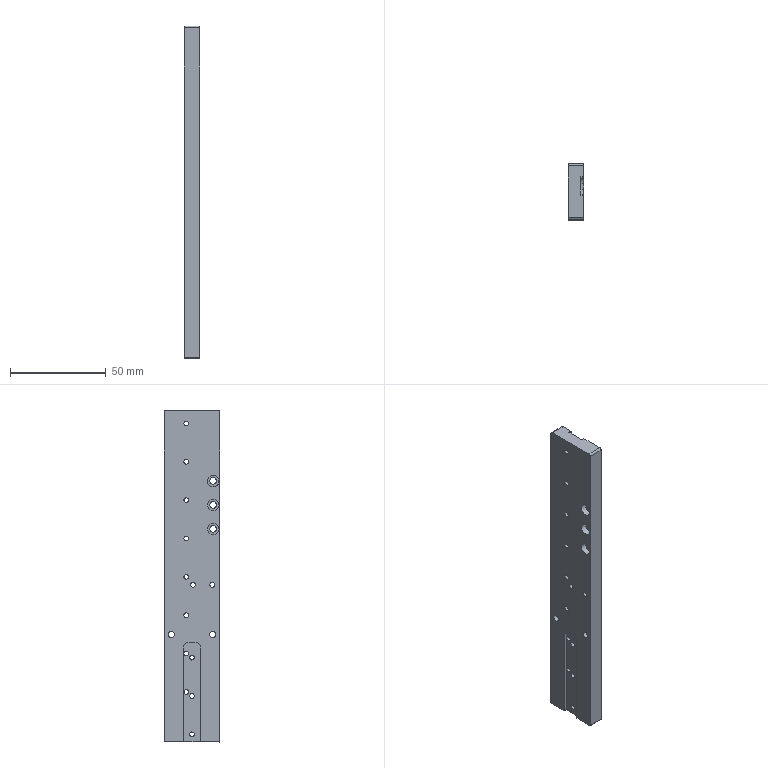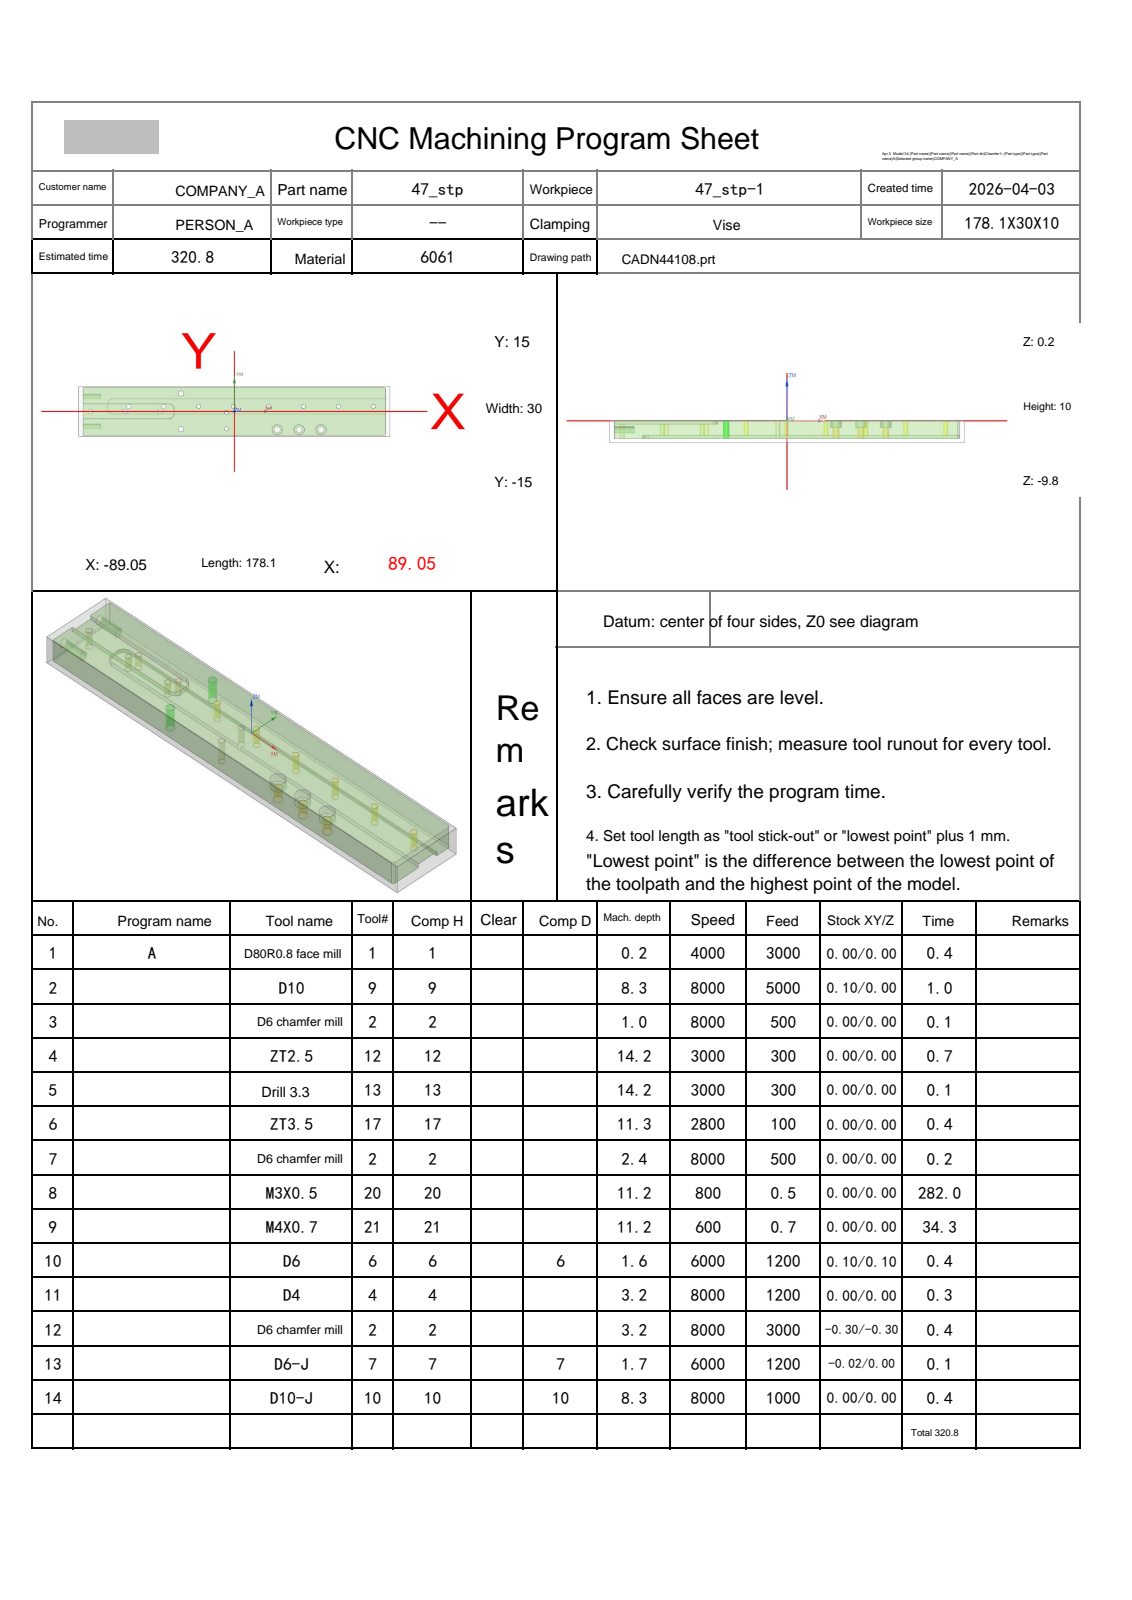NC program | NX | posted by the shop | part box 8 x 29 x 173.1 mm
Whole program:
%
O0001
(Machine time: 611.02 MIN)
(===Total Tool:12===)
(T1=D80R0.8 face mill D=80.  R=0.8  D-  H01 Z=-0.   )
(T9=D10     D=10.  R=0.   D-  H09 Z=-8.1  )
(T2=D6 chamfer mill   D=6.   R=0.   D-  H02 Z=-3.   )
(T12=ZT2.5  D=2.5  DR_a=118 D-  H12 Z=-14.  )
(T13=drill 3.3  D=3.3  DR_a=118 D-  H13 Z=-13.99)
(T17=ZT3.5  D=3.5  DR_a=118 D-  H17 Z=-11.05)
(T20=M3X0.5 D=2.5  DR_a=180 D-  H20 Z=-11.  )
(T21=M4X0.7 D=3.3  DR_a=180 D-  H21 Z=-11.  )
(T6=D6      D=6.   R=0.   D6  H06 Z=-1.4  )
(T4=D4      D=4.   R=0.   D4  H04 Z=-3.   )
(T7=D6-J    D=6.   R=0.   D7  H07 Z=-1.5  )
(T10=D10-J  D=10.  R=0.   D10 H10 Z=-8.1  )
G80 G90 G17 G49 G40
G91 G28 Z0
M01
N1 T01 M06
(D80R0.8 face mill  D=80. R=0.8 H=01 ce=0.20 di=0.10)
G00 G90 G54 X-131.55 Y0.0 M03 S4000
G43 H01 Z20.
M08
Z2.1
G01 Z.1 F3000.
X-126.55
X126.55
X131.55
Z2.1
G00 Z20.
G00 G90 X-131.55 Y0.0 M03 S4000
Z20.
Z2.
G01 Z0.0 F1000.
X-126.55
X126.55
X131.55
Z2.
G00 Z20.
G91 G28 Z0.0
M05
M09
G91 G28 Z0.0
M01
N2 T09 M06
(D10  D=10. R=0. H=09 ce=0.10 di=0.00)
G00 G90 G54 X-.4 Y19.6 M03 S8000
G43 H09 Z20.
M08
Z.5
G01 X85.55 Z.346 F5000.
G02 X91.65 Y13.5 Z.328 I0.0 J-6.1
G01 Y-13.5 Z.28
G02 X85.55 Y-19.6 Z.263 I-6.1 J0.0
G01 X-86.35 Z-.046
G02 X-89.956 Y-18.106 Z-.053 I0.0 J5.1
G01 X-90.156 Y-17.906 Z-.054
G02 X-91.65 Y-14.3 Z-.061 I3.606 J3.606
G01 Y14.3 Z-.112
G02 X-90.156 Y17.906 Z-.12 I5.1 J0.0
G01 X-89.956 Y18.106
G02 X-86.35 Y19.6 Z-.127 I3.606 J-3.606
G01 X85.55 Z-.436
G02 X91.65 Y13.5 Z-.453 I0.0 J-6.1
G01 Y-13.5 Z-.502
G02 X85.55 Y-19.6 Z-.519 I-6.1 J0.0
G01 X-86.35 Z-.828
G02 X-89.956 Y-18.106 Z-.835 I0.0 J5.1
G01 X-90.156 Y-17.906 Z-.836
G02 X-91.65 Y-14.3 Z-.843 I3.606 J3.606
G01 Y14.3 Z-.894
G02 X-90.156 Y17.906 Z-.902 I5.1 J0.0
G01 X-89.956 Y18.106
G02 X-86.35 Y19.6 Z-.909 I3.606 J-3.606
G01 X85.55 Z-1.218
G02 X91.65 Y13.5 Z-1.235 I0.0 J-6.1
G01 Y-13.5 Z-1.284
G02 X85.55 Y-19.6 Z-1.301 I-6.1 J0.0
G01 X-86.35 Z-1.61
G02 X-89.956 Y-18.106 Z-1.617 I0.0 J5.1
G01 X-90.156 Y-17.906 Z-1.618
G02 X-91.65 Y-14.3 Z-1.625 I3.606 J3.606
G01 Y14.3 Z-1.676
G02 X-90.156 Y17.906 Z-1.683 I5.1 J0.0
G01 X-89.956 Y18.106 Z-1.684
G02 X-86.35 Y19.6 Z-1.691 I3.606 J-3.606
G01 X85.55 Z-2.
G02 X91.65 Y13.5 Z-2.017 I0.0 J-6.1
G01 Y-13.5 Z-2.066
G02 X85.55 Y-19.6 Z-2.083 I-6.1 J0.0
G01 X-86.35 Z-2.392
G02 X-89.956 Y-18.106 Z-2.399 I0.0 J5.1
G01 X-90.156 Y-17.906
G02 X-91.65 Y-14.3 Z-2.407 I3.606 J3.606
G01 Y14.3 Z-2.458
G02 X-90.156 Y17.906 Z-2.465 I5.1 J0.0
G01 X-89.956 Y18.106 Z-2.466
G02 X-86.35 Y19.6 Z-2.473 I3.606 J-3.606
G01 X85.55 Z-2.782
G02 X91.65 Y13.5 Z-2.799 I0.0 J-6.1
G01 Y-13.5 Z-2.847
G02 X85.55 Y-19.6 Z-2.865 I-6.1 J0.0
G01 X-86.35 Z-3.173
G02 X-89.956 Y-18.106 Z-3.181 I0.0 J5.1
G01 X-90.156 Y-17.906
G02 X-91.65 Y-14.3 Z-3.188 I3.606 J3.606
G01 Y14.3 Z-3.24
G02 X-90.156 Y17.906 Z-3.247 I5.1 J0.0
G01 X-89.956 Y18.106
G02 X-86.35 Y19.6 Z-3.255 I3.606 J-3.606
G01 X85.55 Z-3.564
G02 X91.65 Y13.5 Z-3.581 I0.0 J-6.1
G01 Y-13.5 Z-3.629
G02 X85.55 Y-19.6 Z-3.646 I-6.1 J0.0
G01 X-86.35 Z-3.955
G02 X-89.956 Y-18.106 Z-3.962 I0.0 J5.1
G01 X-90.156 Y-17.906 Z-3.963
G02 X-91.65 Y-14.3 Z-3.97 I3.606 J3.606
G01 Y14.3 Z-4.022
G02 X-90.156 Y17.906 Z-4.029 I5.1 J0.0
G01 X-89.956 Y18.106
G02 X-86.35 Y19.6 Z-4.036 I3.606 J-3.606
G01 X85.55 Z-4.345
G02 X91.65 Y13.5 Z-4.363 I0.0 J-6.1
G01 Y-13.5 Z-4.411
G02 X85.55 Y-19.6 Z-4.428 I-6.1 J0.0
G01 X-86.35 Z-4.737
G02 X-89.956 Y-18.106 Z-4.744 I0.0 J5.1
G01 X-90.156 Y-17.906 Z-4.745
G02 X-91.65 Y-14.3 Z-4.752 I3.606 J3.606
G01 Y14.3 Z-4.803
G02 X-90.156 Y17.906 Z-4.811 I5.1 J0.0
G01 X-89.956 Y18.106
G02 X-86.35 Y19.6 Z-4.818 I3.606 J-3.606
G01 X85.55 Z-5.127
G02 X91.65 Y13.5 Z-5.144 I0.0 J-6.1
G01 Y-13.5 Z-5.193
G02 X85.55 Y-19.6 Z-5.21 I-6.1 J0.0
G01 X-86.35 Z-5.519
G02 X-89.956 Y-18.106 Z-5.526 I0.0 J5.1
G01 X-90.156 Y-17.906 Z-5.527
G02 X-91.65 Y-14.3 Z-5.534 I3.606 J3.606
G01 Y14.3 Z-5.585
G02 X-90.156 Y17.906 Z-5.592 I5.1 J0.0
G01 X-89.956 Y18.106 Z-5.593
G02 X-86.35 Y19.6 Z-5.6 I3.606 J-3.606
G01 X85.55 Z-5.909
G02 X91.65 Y13.5 Z-5.926 I0.0 J-6.1
G01 Y-13.5 Z-5.975
G02 X85.55 Y-19.6 Z-5.992 I-6.1 J0.0
G01 X-86.35 Z-6.301
G02 X-89.956 Y-18.106 Z-6.308 I0.0 J5.1
G01 X-90.156 Y-17.906
G02 X-91.65 Y-14.3 Z-6.316 I3.606 J3.606
G01 Y14.3 Z-6.367
G02 X-90.156 Y17.906 Z-6.374 I5.1 J0.0
G01 X-89.956 Y18.106 Z-6.375
G02 X-86.35 Y19.6 Z-6.382 I3.606 J-3.606
G01 X85.55 Z-6.691
G02 X91.65 Y13.5 Z-6.708 I0.0 J-6.1
G01 Y-13.5 Z-6.757
G02 X85.55 Y-19.6 Z-6.774 I-6.1 J0.0
G01 X-86.35 Z-7.083
G02 X-89.956 Y-18.106 Z-7.09 I0.0 J5.1
G01 X-90.156 Y-17.906
G02 X-91.65 Y-14.3 Z-7.097 I3.606 J3.606
G01 Y14.3 Z-7.149
G02 X-90.156 Y17.906 Z-7.156 I5.1 J0.0
G01 X-89.956 Y18.106 Z-7.157
G02 X-86.35 Y19.6 Z-7.164 I3.606 J-3.606
G01 X85.55 Z-7.473
G02 X91.65 Y13.5 Z-7.49 I0.0 J-6.1
G01 Y-13.5 Z-7.538
G02 X85.55 Y-19.6 Z-7.556 I-6.1 J0.0
G01 X-86.35 Z-7.864
G02 X-89.956 Y-18.106 Z-7.872 I0.0 J5.1
G01 X-90.156 Y-17.906
G02 X-91.65 Y-14.3 Z-7.879 I3.606 J3.606
G01 Y14.3 Z-7.931
G02 X-90.156 Y17.906 Z-7.938 I5.1 J0.0
G01 X-89.956 Y18.106
G02 X-86.35 Y19.6 Z-7.946 I3.606 J-3.606
G01 X-.4 Z-8.1
X85.55
G02 X91.65 Y13.5 I0.0 J-6.1
G01 Y-13.5
G02 X85.55 Y-19.6 I-6.1 J0.0
G01 X-86.35
G02 X-89.956 Y-18.106 I0.0 J5.1
G01 X-90.156 Y-17.906
G02 X-91.65 Y-14.3 I3.606 J3.606
G01 Y14.3
G02 X-90.156 Y17.906 I5.1 J0.0
G01 X-89.956 Y18.106
G02 X-86.35 Y19.6 I3.606 J-3.606
G01 X-.4
X.1
Z-7.1
G00 Z20.
G91 G28 Z0.0
M05
M09
G91 G28 Z0.0
M01
N3 T02 M06
(D6 chamfer mill  D=6. R=0. H=02 ce=0.00 di=0.00)
G00 G90 G54 X-82.55 Y0.0 M03 S8000
G43 H02 Z20.
M08
G98 G81 X-82.55 Y0.0 Z-.8 R1. F500.
X-62.55
X-60.45 Y3.
X-42.55 Y0.0
X-40.45 Y3.
X-30.55 Y10.75
X-20.45 Y3.
X-30.55 Y-10.75
X-4.574 Y-10.55
Y-.55
X-.45 Y3.
X19.55
X24.55 Y-11.045
X37.05
X39.55 Y3.
X49.55 Y-11.045
X59.55 Y3.
X79.55
G80
G00 Z20.
G91 G28 Z0.0
M05
M09
G91 G28 Z0.0
M01
N4 T12 M06
(ZT2.5 D=2.5 DR_a=118 H=12)
G00 G90 G54 X-82.55 Y0.0 M03 S3000
G43 H12 Z20.
M08
G98 G83 X-82.55 Y0.0 Z-14. R1. F300. Q2.
X-62.55
X-60.45 Y3.
X-42.55 Y0.0
X-40.45 Y3.
X-20.45
X-4.574 Y-10.55
Y-.55
X-.45 Y3.
X19.55
X39.55
X59.55
X79.55
G80
G00 Z20.
G91 G28 Z0.0
M05
M09
G91 G28 Z0.0
M01
N5 T13 M06
(drill 3.3 D=3.3 DR_a=118 H=13)
G00 G90 G54 X-30.55 Y10.75 M03 S3000
G43 H13 Z20.
M08
G98 G83 X-30.55 Y10.75 Z-13.991 R1. F300. Q2.
Y-10.75
G80
G00 Z20.
G91 G28 Z0.0
M05
M09
G91 G28 Z0.0
M01
N6 T17 M06
(ZT3.5 D=3.5 DR_a=118 H=17)
G00 G90 G54 X49.55 Y-11.045 M03 S2800
G43 H17 Z20.
M08
G98 G83 X49.55 Y-11.045 Z-11.052 R1. F100. Q2.
X37.05
X24.55
G80
G00 Z20.
G91 G28 Z0.0
M05
M09
G91 G28 Z0.0
M01
N7 T02 M06
(D6 chamfer mill  D=6. R=0. H=02 ce=0.00 di=0.00)
G00 G90 G54 X-82.55 Y0.0 M03 S8000
G43 H02 Z20.
M08
G98 G81 X-82.55 Y0.0 Z-1.75 R3. F500.
X-62.55
X-60.45 Y3.
X-42.55 Y0.0
X-40.45 Y3.
X-20.45
X-4.574 Y-10.55
Y-.55
X-.45 Y3.
X19.55
X39.55
X59.55
X79.55
G80
G00 Z20.
G00 G90 X-30.55 Y10.75 M03 S8000
Z20.
G98 G81 X-30.55 Y10.75 Z-2.2 R3. F500.
Y-10.75
G80
G00 Z20.
G91 G28 Z0.0
M05
M09
G91 G28 Z0.0
M01
N8 T20 M06
(M3X0.5 D=2.5 DR_a=180 H=20)
G00 G90 G54 X-82.55 Y0.0 M03 S800
G43 H20 Z20.
M08
G95
G98 G84 X-82.55 Y0.0 Z-11. R1. F.5 Q5.
G98 G84 X-62.55 Y0.0 Z-9.5 R1.
X-60.45 Y3.
X-42.55 Y0.0
X-40.45 Y3.
X-20.45
G98 G84 X-4.574 Y-10.55 Z-11. R1.
Y-.55
G98 G84 X-.45 Y3. Z-9.5 R1.
X19.55
X39.55
X59.55
X79.55
G80
G94
G00 Z20.
G91 G28 Z0.0
M05
M09
G91 G28 Z0.0
M01
N9 T21 M06
(M4X0.7 D=3.3 DR_a=180 H=21)
G00 G90 G54 X-30.55 Y10.75 M03 S600
G43 H21 Z20.
M08
G95
G98 G84 X-30.55 Y10.75 Z-11. R1. F.7 Q4.
Y-10.75
G80
G94
G00 Z20.
G91 G28 Z0.0
M05
M09
G91 G28 Z0.0
M01
N10 T06 M06
(D6  D=6. R=0. H=06 ce=0.10 di=0.10)
G00 G90 G54 X-90.746 Y-3.671 M03 S6000
G43 H06 Z20.
M08
Z.15
G01 Z-.35 F1200.
G41 D06
X-90.65 Y-3.7
G03 X-90.357 Y-3.744 I.293 J.956
X-89.65 Y-3.451 I0.0 J1.
G01 X-87.634 Y-1.435
X-37.615
Y1.435
X-87.634
X-89.65 Y3.451
G03 X-90.357 Y3.744 I-.707 J-.707
X-90.65 Y3.7 I0.0 J-1.
G01 G40 X-90.746 Y3.671
Z.15
G00 Z20.
Y-3.671
Z-.2
G01 Z-.7
G41 D06
X-90.65 Y-3.7
G03 X-90.357 Y-3.744 I.293 J.956
X-89.65 Y-3.451 I0.0 J1.
G01 X-87.634 Y-1.435
X-37.615
Y1.435
X-87.634
X-89.65 Y3.451
G03 X-90.357 Y3.744 I-.707 J-.707
X-90.65 Y3.7 I0.0 J-1.
G01 G40 X-90.746 Y3.671
Z-.2
G00 Z20.
Y-3.671
Z-.55
G01 Z-1.05
G41 D06
X-90.65 Y-3.7
G03 X-90.357 Y-3.744 I.293 J.956
X-89.65 Y-3.451 I0.0 J1.
G01 X-87.634 Y-1.435
X-37.615
Y1.435
X-87.634
X-89.65 Y3.451
G03 X-90.357 Y3.744 I-.707 J-.707
X-90.65 Y3.7 I0.0 J-1.
G01 G40 X-90.746 Y3.671
Z-.55
G00 Z20.
Y-3.671
Z-.9
G01 Z-1.4
G41 D06
X-90.65 Y-3.7
G03 X-90.357 Y-3.744 I.293 J.956
X-89.65 Y-3.451 I0.0 J1.
G01 X-87.634 Y-1.435
X-37.615
Y1.435
X-87.634
X-89.65 Y3.451
G03 X-90.357 Y3.744 I-.707 J-.707
X-90.65 Y3.7 I0.0 J-1.
G01 G40 X-90.746 Y3.671
Z-.9
G00 Z20.
G91 G28 Z0.0
M05
M09
G91 G28 Z0.0
M01
N11 T04 M06
(D4  D=4. R=0. H=04 ce=0.10 di=0.00)
G00 G90 G54 X49.55 Y-11.045 M03 S8000
G43 H04 Z20.
M08
Z.5
G03 X50. Y-10.595 I0.0 J.45 F1200.
X49.55 Y-10.145 I-.45 J0.0
X49.55 Y-10.145 Z.2 I0.0 J-.9
X49.55 Y-10.145 Z-.1 I0.0 J-.9
X49.55 Y-10.145 Z-.4 I0.0 J-.9
X49.55 Y-10.145 Z-.7 I0.0 J-.9
X49.55 Y-10.145 Z-1. I0.0 J-.9
X49.55 Y-10.145 Z-1.3 I0.0 J-.9
X49.55 Y-10.145 Z-1.6 I0.0 J-.9
X49.55 Y-10.145 Z-1.9 I0.0 J-.9
X49.55 Y-10.145 Z-2.2 I0.0 J-.9
X49.55 Y-10.145 Z-2.5 I0.0 J-.9
X49.55 Y-10.145 Z-2.8 I0.0 J-.9
X50.329 Y-11.495 Z-3. I0.0 J-.9
X50.45 Y-11.045 I-.779 J.45
X49.55 Y-10.145 I-.9 J0.0
X48.65 Y-11.045 I0.0 J-.9
X49.55 Y-11.945 I.9 J0.0
X50.329 Y-11.495 I0.0 J.9
X50.39 Y-11.27 I-.39 J.225
X49.94 Y-10.82 I-.45 J0.0
X49.55 Y-11.045 I0.0 J-.45
G00 Z20.
X37.05
Z.5
G03 X37.5 Y-10.595 I0.0 J.45
X37.05 Y-10.145 I-.45 J0.0
X37.05 Y-10.145 Z.2 I0.0 J-.9
X37.05 Y-10.145 Z-.1 I0.0 J-.9
X37.05 Y-10.145 Z-.4 I0.0 J-.9
X37.05 Y-10.145 Z-.7 I0.0 J-.9
X37.05 Y-10.145 Z-1. I0.0 J-.9
X37.05 Y-10.145 Z-1.3 I0.0 J-.9
X37.05 Y-10.145 Z-1.6 I0.0 J-.9
X37.05 Y-10.145 Z-1.9 I0.0 J-.9
X37.05 Y-10.145 Z-2.2 I0.0 J-.9
X37.05 Y-10.145 Z-2.5 I0.0 J-.9
X37.05 Y-10.145 Z-2.8 I0.0 J-.9
X37.829 Y-11.495 Z-3. I0.0 J-.9
X37.95 Y-11.045 I-.779 J.45
X37.05 Y-10.145 I-.9 J0.0
X36.15 Y-11.045 I0.0 J-.9
X37.05 Y-11.945 I.9 J0.0
X37.829 Y-11.495 I0.0 J.9
X37.89 Y-11.27 I-.39 J.225
X37.44 Y-10.82 I-.45 J0.0
X37.05 Y-11.045 I0.0 J-.45
G00 Z20.
X24.55
Z.5
G03 X25. Y-10.595 I0.0 J.45
X24.55 Y-10.145 I-.45 J0.0
X24.55 Y-10.145 Z.2 I0.0 J-.9
X24.55 Y-10.145 Z-.1 I0.0 J-.9
X24.55 Y-10.145 Z-.4 I0.0 J-.9
X24.55 Y-10.145 Z-.7 I0.0 J-.9
X24.55 Y-10.145 Z-1. I0.0 J-.9
X24.55 Y-10.145 Z-1.3 I0.0 J-.9
X24.55 Y-10.145 Z-1.6 I0.0 J-.9
X24.55 Y-10.145 Z-1.9 I0.0 J-.9
X24.55 Y-10.145 Z-2.2 I0.0 J-.9
X24.55 Y-10.145 Z-2.5 I0.0 J-.9
X24.55 Y-10.145 Z-2.8 I0.0 J-.9
X25.329 Y-11.495 Z-3. I0.0 J-.9
X25.45 Y-11.045 I-.779 J.45
X24.55 Y-10.145 I-.9 J0.0
X23.65 Y-11.045 I0.0 J-.9
X24.55 Y-11.945 I.9 J0.0
X25.329 Y-11.495 I0.0 J.9
X25.39 Y-11.27 I-.39 J.225
X24.94 Y-10.82 I-.45 J0.0
X24.55 Y-11.045 I0.0 J-.45
G00 Z20.
G00 G90 X49.55 Y-11.045 M03 S8000
Z20.
Z.5
G41 D04
G01 X49.735 Y-10.968 F500.
G03 X50.03 Y-10.525 I-.185 J.443
X49.55 Y-10.045 I-.48 J0.0
X50.501 Y-11.354 Z-3. I0.0 J-1.
X50.55 Y-11.045 I-.951 J.309
X49.55 Y-10.045 I-1. J0.0
X48.55 Y-11.045 I0.0 J-1.
X49.55 Y-12.045 I1. J0.0
X50.501 Y-11.354 I0.0 J1.
G01 X50.525 Y-11.206
G03 X50.045 Y-10.726 I-.48 J0.0
X49.68 Y-10.893 I0.0 J-.48
G01 G40 X49.55 Y-11.045
G00 Z20.
X37.05
Z.5
G41 D04
G01 X37.235 Y-10.968
G03 X37.53 Y-10.525 I-.185 J.443
X37.05 Y-10.045 I-.48 J0.0
X38.001 Y-11.354 Z-3. I0.0 J-1.
X38.05 Y-11.045 I-.951 J.309
X37.05 Y-10.045 I-1. J0.0
X36.05 Y-11.045 I0.0 J-1.
X37.05 Y-12.045 I1. J0.0
X38.001 Y-11.354 I0.0 J1.
G01 X38.025 Y-11.206
G03 X37.545 Y-10.726 I-.48 J0.0
X37.18 Y-10.893 I0.0 J-.48
G01 G40 X37.05 Y-11.045
G00 Z20.
X24.55
Z.5
G41 D04
G01 X24.735 Y-10.968
G03 X25.03 Y-10.525 I-.185 J.443
X24.55 Y-10.045 I-.48 J0.0
X25.501 Y-11.354 Z-3. I0.0 J-1.
X25.55 Y-11.045 I-.951 J.309
X24.55 Y-10.045 I-1. J0.0
X23.55 Y-11.045 I0.0 J-1.
X24.55 Y-12.045 I1. J0.0
X25.501 Y-11.354 I0.0 J1.
G01 X25.525 Y-11.206
G03 X25.045 Y-10.726 I-.48 J0.0
X24.68 Y-10.893 I0.0 J-.48
G01 G40 X24.55 Y-11.045
G00 Z20.
G91 G28 Z0.0
M05
M09
G91 G28 Z0.0
M01
N12 T02 M06
(D6 chamfer mill  D=6. R=0. H=02 ce=-0.30 di=0.00)
G00 G90 G54 X25.72 Y-13.026 M03 S8000
G43 H02 Z20.
M08
Z2.5
G01 X25.802 Y-12.978 Z2.465 F500.
X26.063 Y-12.781 Z2.346
X26.294 Y-12.549 Z2.227
X26.49 Y-12.286 Z2.108
X26.646 Y-11.999 Z1.989
X26.76 Y-11.692 Z1.87
X26.83 Y-11.372 Z1.75
X26.853 Y-11.045 Z1.631
X26.83 Y-10.718 Z1.512
X26.76 Y-10.398 Z1.393
X26.646 Y-10.091 Z1.274
X26.49 Y-9.804 Z1.154
X26.294 Y-9.541 Z1.035
X26.063 Y-9.309 Z.916
X25.802 Y-9.112 Z.797
X25.598 Y-8.994 Z.711
X25.297 Y-8.866 Z.592
X24.98 Y-8.783 Z.473
X24.655 Y-8.744 Z.354
X24.328 Y-8.753 Z.235
X24.005 Y-8.807 Z.115
X23.693 Y-8.907 Z-.004
X23.399 Y-9.051 Z-.123
X23.127 Y-9.234 Z-.242
X22.885 Y-9.454 Z-.361
X22.676 Y-9.706 Z-.48
X22.505 Y-9.986 Z-.6
X22.376 Y-10.286 Z-.719
X22.29 Y-10.602 Z-.838
X22.25 Y-10.927 Z-.957
Y-11.045 Z-1.
G03 X24.55 Y-13.345 I2.3 J0.0
X26.85 Y-11.045 I0.0 J2.3
X24.55 Y-8.745 I-2.3 J0.0
X22.25 Y-11.045 I0.0 J-2.3
X22.304 Y-11.541 I2.3 J0.0
G01 Z1.5
G00 Z20.
X38.22 Y-13.026
Z2.5
G01 X38.302 Y-12.978 Z2.465
X38.563 Y-12.781 Z2.346
X38.794 Y-12.549 Z2.227
X38.99 Y-12.286 Z2.108
X39.146 Y-11.999 Z1.989
X39.26 Y-11.692 Z1.87
X39.33 Y-11.372 Z1.75
X39.353 Y-11.045 Z1.631
X39.33 Y-10.718 Z1.512
X39.26 Y-10.398 Z1.393
X39.146 Y-10.091 Z1.274
X38.99 Y-9.804 Z1.154
X38.794 Y-9.541 Z1.035
X38.563 Y-9.309 Z.916
X38.302 Y-9.112 Z.797
X38.098 Y-8.994 Z.711
X37.797 Y-8.866 Z.592
X37.48 Y-8.783 Z.473
X37.155 Y-8.744 Z.354
X36.828 Y-8.753 Z.235
X36.505 Y-8.807 Z.115
X36.193 Y-8.907 Z-.004
X35.899 Y-9.051 Z-.123
X35.627 Y-9.234 Z-.242
X35.385 Y-9.454 Z-.361
X35.176 Y-9.706 Z-.48
X35.005 Y-9.986 Z-.6
X34.876 Y-10.286 Z-.719
X34.79 Y-10.602 Z-.838
X34.75 Y-10.927 Z-.957
Y-11.045 Z-1.
G03 X37.05 Y-13.345 I2.3 J0.0
X39.35 Y-11.045 I0.0 J2.3
X37.05 Y-8.745 I-2.3 J0.0
X34.75 Y-11.045 I0.0 J-2.3
X34.804 Y-11.541 I2.3 J0.0
G01 Z1.5
G00 Z20.
X50.72 Y-13.026
Z2.5
G01 X50.802 Y-12.978 Z2.465
X51.063 Y-12.781 Z2.346
X51.294 Y-12.549 Z2.227
X51.49 Y-12.286 Z2.108
X51.646 Y-11.999 Z1.989
X51.76 Y-11.692 Z1.87
X51.83 Y-11.372 Z1.75
X51.853 Y-11.045 Z1.631
X51.83 Y-10.718 Z1.512
X51.76 Y-10.398 Z1.393
X51.646 Y-10.091 Z1.274
X51.49 Y-9.804 Z1.154
X51.294 Y-9.541 Z1.035
X51.063 Y-9.309 Z.916
X50.802 Y-9.112 Z.797
X50.598 Y-8.994 Z.711
X50.297 Y-8.866 Z.592
X49.98 Y-8.783 Z.473
X49.655 Y-8.744 Z.354
X49.328 Y-8.753 Z.235
X49.005 Y-8.807 Z.115
X48.693 Y-8.907 Z-.004
X48.399 Y-9.051 Z-.123
X48.127 Y-9.234 Z-.242
X47.885 Y-9.454 Z-.361
X47.676 Y-9.706 Z-.48
X47.505 Y-9.986 Z-.6
X47.376 Y-10.286 Z-.719
X47.29 Y-10.602 Z-.838
X47.25 Y-10.927 Z-.957
Y-11.045 Z-1.
G03 X49.55 Y-13.345 I2.3 J0.0
X51.85 Y-11.045 I0.0 J2.3
X49.55 Y-8.745 I-2.3 J0.0
X47.25 Y-11.045 I0.0 J-2.3
X47.304 Y-11.541 I2.3 J0.0
G01 Z1.5
G00 Z20.
G00 G90 X-.15 Y-16.628 M03 S8000
Z20.
Z2.099
G01 Z-1.5 F3000.
G03 X-.07 Y-16.328 I-.52 J.3
X-.37 Y-15.808 I-.6 J0.0
G01 X-.4 Y-15.8
X-86.35
X-86.604 Y-15.775
X-86.847 Y-15.701
X-87.072 Y-15.581
X-87.269 Y-15.419
X-87.469 Y-15.219
X-87.631 Y-15.022
X-87.751 Y-14.797
X-87.825 Y-14.554
X-87.85 Y-14.3
Y-4.735
X-87.825 Y-4.481
X-87.751 Y-4.238
X-87.631 Y-4.013
X-87.469 Y-3.816
X-87.269 Y-3.616
X-87.072 Y-3.454
X-86.847 Y-3.334
X-86.604 Y-3.26
X-86.35 Y-3.235
X-37.55
G03 X-35.815 Y-1.5 I0.0 J1.735
G01 Y1.5
G03 X-37.55 Y3.235 I-1.735 J0.0
G01 X-86.35
X-86.604 Y3.26
X-86.847 Y3.334
X-87.072 Y3.454
X-87.269 Y3.616
X-87.469 Y3.816
X-87.631 Y4.013
X-87.751 Y4.238
X-87.825 Y4.481
X-87.85 Y4.735
Y14.3
X-87.825 Y14.554
X-87.751 Y14.797
X-87.631 Y15.022
X-87.469 Y15.219
X-87.269 Y15.419
X-87.072 Y15.581
X-86.848 Y15.701
X-86.604 Y15.775
X-86.35 Y15.8
X85.55
G02 X87.85 Y13.5 I0.0 J-2.3
G01 Y-13.5
G02 X85.55 Y-15.8 I-2.3 J0.0
G01 X-.4
X-.43 Y-15.808
G03 X-.73 Y-16.328 I.3 J-.52
X-.65 Y-16.628 I.6 J0.0
G01 Z2.099
G00 Z20.
X-87.85 Y-1.961
Z1.755
G01 Z-3.
Y1.961
Z1.755
G00 Z20.
G91 G28 Z0.0
M05
M09
G91 G28 Z0.0
M01
N13 T07 M06
(D6-J  D=6. R=0. H=07 ce=-0.02 di=0.00)
G00 G90 G54 X-90.63 Y-6.573 M03 S6000
G43 H07 Z20.
M08
Z-1.
G01 Z-1.5 F1200.
G41 D07
X-90.53
G03 X-89.53 Y-5.573 I0.0 J1.
G01 Y-3.501
X-87.584 Y-1.555
X-37.55
X-37.518 Y-1.556
X-37.494 Y-1.533
X-37.495 Y-1.5
Y1.5
X-37.494 Y1.533
X-37.518 Y1.556
X-37.55 Y1.555
X-87.584
X-89.53 Y3.501
Y5.573
G03 X-90.53 Y6.573 I-1. J0.0
G01 G40 X-90.63
Z-1.
G00 Z20.
G91 G28 Z0.0
M05
M09
G91 G28 Z0.0
M01
N14 T10 M06
(D10-J  D=10. R=0. H=10 ce=0.00 di=0.00)
G00 G90 G54 X-87.363 Y20.616 M03 S8000
G43 H10 Z20.
M08
Z-7.6
G01 Z-8.1 F1000.
G41 D10
X-87.347 Y20.417
G03 X-86.35 Y19.5 I.997 J.083
G01 X85.55
G02 X91.55 Y13.5 I0.0 J-6.
G01 Y-1.735
Y-13.5
G02 X85.55 Y-19.5 I-6. J0.0
G01 X-86.35
G02 X-89.886 Y-18.036 I0.0 J5.
G01 X-90.086 Y-17.836
G02 X-91.55 Y-14.3 I3.536 J3.536
G01 Y14.3
G02 X-90.086 Y17.836 I5. J0.0
G01 X-89.886 Y18.036
G02 X-86.35 Y19.5 I3.536 J-3.536
G01 X-85.85
G03 X-84.85 Y20.5 I0.0 J1.
G01 G40 Y20.7
Z-7.6
G00 Z20.
M05
M09
G91 G28 Z0.0
G91 G28 Y0.0
M30
%